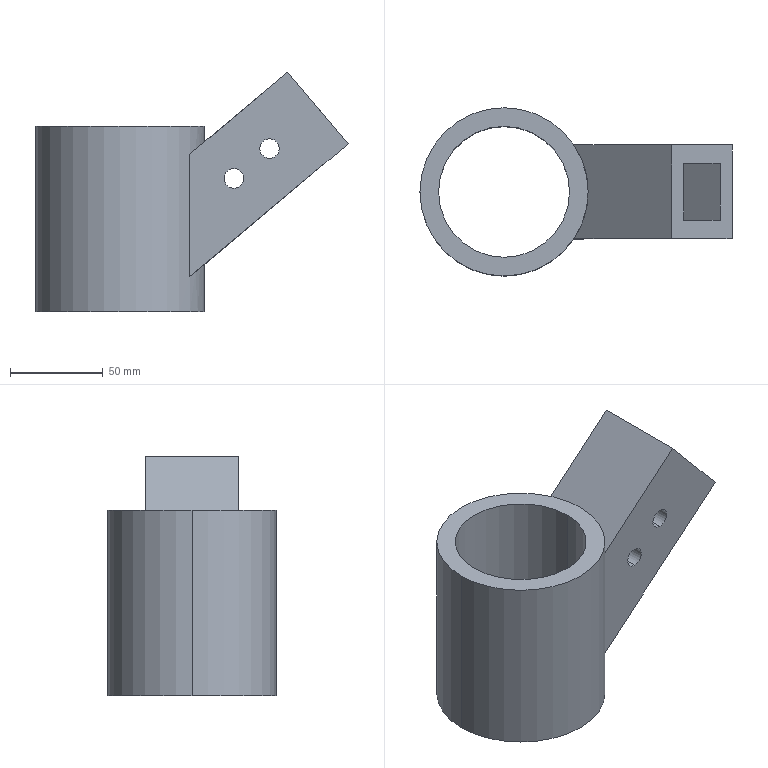Part | SolidWorks | features MirrorStock 1 | 1 solid | 24 faces | box 167.949 x 90.5 x 129.102 mm | volume 386069 mm3 | cylinder 13 | plane 11 | commonest cylinder face diameters 10.5 x8 90.5 x3 70.5 x2
STEP:
#1=CARTESIAN_POINT('',(80.423,15.25,43.155));
#2=VERTEX_POINT('',#1);
#3=CARTESIAN_POINT('',(80.423,15.25,32.655));
#4=VERTEX_POINT('',#3);
#5=CARTESIAN_POINT('',(80.423,15.25,37.905));
#6=DIRECTION('',(0.,1.,0.));
#7=DIRECTION('',(0.,0.,1.));
#8=AXIS2_PLACEMENT_3D('',#5,#6,#7);
#9=CIRCLE('',#8,5.25);
#10=EDGE_CURVE('',#2,#4,#9,.T.);
#11=ORIENTED_EDGE('',*,*,#10,.F.);
#12=CARTESIAN_POINT('',(80.423,25.25,43.155));
#13=VERTEX_POINT('',#12);
#14=CARTESIAN_POINT('',(80.423,-57.25,43.155));
#15=DIRECTION('',(0.,1.,0.));
#16=VECTOR('',#15,1000.);
#17=LINE('',#14,#16);
#18=EDGE_CURVE('',#2,#13,#17,.T.);
#19=ORIENTED_EDGE('',*,*,#18,.T.);
#20=CARTESIAN_POINT('',(80.423,25.25,32.655));
#21=VERTEX_POINT('',#20);
#22=CARTESIAN_POINT('',(80.423,25.25,37.905));
#23=DIRECTION('',(0.,1.,0.));
#24=DIRECTION('',(0.,0.,1.));
#25=AXIS2_PLACEMENT_3D('',#22,#23,#24);
#26=CIRCLE('',#25,5.25);
#27=EDGE_CURVE('',#13,#21,#26,.T.);
#28=ORIENTED_EDGE('',*,*,#27,.T.);
#29=CARTESIAN_POINT('',(80.423,-57.25,32.655));
#30=DIRECTION('',(0.,1.,0.));
#31=VECTOR('',#30,1000.);
#32=LINE('',#29,#31);
#33=EDGE_CURVE('',#4,#21,#32,.T.);
#34=ORIENTED_EDGE('',*,*,#33,.F.);
#35=EDGE_LOOP('',(#11,#19,#28,#34));
#36=FACE_OUTER_BOUND('',#35,.T.);
#37=CARTESIAN_POINT('',(80.423,-57.25,37.905));
#38=DIRECTION('',(0.,1.,0.));
#39=DIRECTION('',(0.,0.,-1.));
#40=AXIS2_PLACEMENT_3D('',#37,#38,#39);
#41=CYLINDRICAL_SURFACE('',#40,5.25);
#42=ADVANCED_FACE('',(#36),#41,.F.);
#43=CARTESIAN_POINT('',(61.272,15.25,27.085));
#44=VERTEX_POINT('',#43);
#45=CARTESIAN_POINT('',(61.272,15.25,16.585));
#46=VERTEX_POINT('',#45);
#47=CARTESIAN_POINT('',(61.272,15.25,21.835));
#48=DIRECTION('',(0.,1.,0.));
#49=DIRECTION('',(0.,0.,1.));
#50=AXIS2_PLACEMENT_3D('',#47,#48,#49);
#51=CIRCLE('',#50,5.25);
#52=EDGE_CURVE('',#44,#46,#51,.T.);
#53=ORIENTED_EDGE('',*,*,#52,.F.);
#54=CARTESIAN_POINT('',(61.272,25.25,27.085));
#55=VERTEX_POINT('',#54);
#56=CARTESIAN_POINT('',(61.272,-57.25,27.085));
#57=DIRECTION('',(0.,1.,0.));
#58=VECTOR('',#57,1000.);
#59=LINE('',#56,#58);
#60=EDGE_CURVE('',#44,#55,#59,.T.);
#61=ORIENTED_EDGE('',*,*,#60,.T.);
#62=CARTESIAN_POINT('',(61.272,25.25,16.585));
#63=VERTEX_POINT('',#62);
#64=CARTESIAN_POINT('',(61.272,25.25,21.835));
#65=DIRECTION('',(0.,1.,0.));
#66=DIRECTION('',(0.,0.,1.));
#67=AXIS2_PLACEMENT_3D('',#64,#65,#66);
#68=CIRCLE('',#67,5.25);
#69=EDGE_CURVE('',#55,#63,#68,.T.);
#70=ORIENTED_EDGE('',*,*,#69,.T.);
#71=CARTESIAN_POINT('',(61.272,-57.25,16.585));
#72=DIRECTION('',(0.,1.,0.));
#73=VECTOR('',#72,1000.);
#74=LINE('',#71,#73);
#75=EDGE_CURVE('',#46,#63,#74,.T.);
#76=ORIENTED_EDGE('',*,*,#75,.F.);
#77=EDGE_LOOP('',(#53,#61,#70,#76));
#78=FACE_OUTER_BOUND('',#77,.T.);
#79=CARTESIAN_POINT('',(61.272,-57.25,21.835));
#80=DIRECTION('',(0.,1.,0.));
#81=DIRECTION('',(0.,0.,-1.));
#82=AXIS2_PLACEMENT_3D('',#79,#80,#81);
#83=CYLINDRICAL_SURFACE('',#82,5.25);
#84=ADVANCED_FACE('',(#78),#83,.F.);
#85=CARTESIAN_POINT('',(80.423,-25.25,32.655));
#86=VERTEX_POINT('',#85);
#87=CARTESIAN_POINT('',(80.423,-25.25,43.155));
#88=VERTEX_POINT('',#87);
#89=CARTESIAN_POINT('',(80.423,-25.25,37.905));
#90=DIRECTION('',(0.,-1.,0.));
#91=DIRECTION('',(0.,0.,-1.));
#92=AXIS2_PLACEMENT_3D('',#89,#90,#91);
#93=CIRCLE('',#92,5.25);
#94=EDGE_CURVE('',#86,#88,#93,.T.);
#95=ORIENTED_EDGE('',*,*,#94,.T.);
#96=CARTESIAN_POINT('',(80.423,-15.25,43.155));
#97=VERTEX_POINT('',#96);
#98=CARTESIAN_POINT('',(80.423,-57.25,43.155));
#99=DIRECTION('',(0.,1.,0.));
#100=VECTOR('',#99,1000.);
#101=LINE('',#98,#100);
#102=EDGE_CURVE('',#88,#97,#101,.T.);
#103=ORIENTED_EDGE('',*,*,#102,.T.);
#104=CARTESIAN_POINT('',(80.423,-15.25,32.655));
#105=VERTEX_POINT('',#104);
#106=CARTESIAN_POINT('',(80.423,-15.25,37.905));
#107=DIRECTION('',(0.,-1.,0.));
#108=DIRECTION('',(0.,0.,-1.));
#109=AXIS2_PLACEMENT_3D('',#106,#107,#108);
#110=CIRCLE('',#109,5.25);
#111=EDGE_CURVE('',#105,#97,#110,.T.);
#112=ORIENTED_EDGE('',*,*,#111,.F.);
#113=CARTESIAN_POINT('',(80.423,-57.25,32.655));
#114=DIRECTION('',(0.,1.,0.));
#115=VECTOR('',#114,1000.);
#116=LINE('',#113,#115);
#117=EDGE_CURVE('',#86,#105,#116,.T.);
#118=ORIENTED_EDGE('',*,*,#117,.F.);
#119=EDGE_LOOP('',(#95,#103,#112,#118));
#120=FACE_OUTER_BOUND('',#119,.T.);
#121=CARTESIAN_POINT('',(80.423,-57.25,37.905));
#122=DIRECTION('',(0.,1.,0.));
#123=DIRECTION('',(0.,0.,-1.));
#124=AXIS2_PLACEMENT_3D('',#121,#122,#123);
#125=CYLINDRICAL_SURFACE('',#124,5.25);
#126=ADVANCED_FACE('',(#120),#125,.F.);
#127=CARTESIAN_POINT('',(61.272,-25.25,16.585));
#128=VERTEX_POINT('',#127);
#129=CARTESIAN_POINT('',(61.272,-25.25,27.085));
#130=VERTEX_POINT('',#129);
#131=CARTESIAN_POINT('',(61.272,-25.25,21.835));
#132=DIRECTION('',(0.,-1.,0.));
#133=DIRECTION('',(0.,0.,-1.));
#134=AXIS2_PLACEMENT_3D('',#131,#132,#133);
#135=CIRCLE('',#134,5.25);
#136=EDGE_CURVE('',#128,#130,#135,.T.);
#137=ORIENTED_EDGE('',*,*,#136,.T.);
#138=CARTESIAN_POINT('',(61.272,-15.25,27.085));
#139=VERTEX_POINT('',#138);
#140=CARTESIAN_POINT('',(61.272,-57.25,27.085));
#141=DIRECTION('',(0.,1.,0.));
#142=VECTOR('',#141,1000.);
#143=LINE('',#140,#142);
#144=EDGE_CURVE('',#130,#139,#143,.T.);
#145=ORIENTED_EDGE('',*,*,#144,.T.);
#146=CARTESIAN_POINT('',(61.272,-15.25,16.585));
#147=VERTEX_POINT('',#146);
#148=CARTESIAN_POINT('',(61.272,-15.25,21.835));
#149=DIRECTION('',(0.,-1.,0.));
#150=DIRECTION('',(0.,0.,-1.));
#151=AXIS2_PLACEMENT_3D('',#148,#149,#150);
#152=CIRCLE('',#151,5.25);
#153=EDGE_CURVE('',#147,#139,#152,.T.);
#154=ORIENTED_EDGE('',*,*,#153,.F.);
#155=CARTESIAN_POINT('',(61.272,-57.25,16.585));
#156=DIRECTION('',(0.,1.,0.));
#157=VECTOR('',#156,1000.);
#158=LINE('',#155,#157);
#159=EDGE_CURVE('',#128,#147,#158,.T.);
#160=ORIENTED_EDGE('',*,*,#159,.F.);
#161=EDGE_LOOP('',(#137,#145,#154,#160));
#162=FACE_OUTER_BOUND('',#161,.T.);
#163=CARTESIAN_POINT('',(61.272,-57.25,21.835));
#164=DIRECTION('',(0.,1.,0.));
#165=DIRECTION('',(0.,0.,-1.));
#166=AXIS2_PLACEMENT_3D('',#163,#164,#165);
#167=CYLINDRICAL_SURFACE('',#166,5.25);
#168=ADVANCED_FACE('',(#162),#167,.F.);
#169=CARTESIAN_POINT('',(35.25,0.,-50.));
#170=VERTEX_POINT('',#169);
#171=CARTESIAN_POINT('',(-35.25,0.,-50.));
#172=VERTEX_POINT('',#171);
#173=CARTESIAN_POINT('',(0.,0.,-50.));
#174=DIRECTION('',(0.,0.,1.));
#175=DIRECTION('',(1.,0.,0.));
#176=AXIS2_PLACEMENT_3D('',#173,#174,#175);
#177=CIRCLE('',#176,35.25);
#178=EDGE_CURVE('',#170,#172,#177,.T.);
#179=ORIENTED_EDGE('',*,*,#178,.F.);
#180=CARTESIAN_POINT('',(35.25,0.,50.));
#181=VERTEX_POINT('',#180);
#182=CARTESIAN_POINT('',(35.25,0.,-50.));
#183=DIRECTION('',(0.,0.,1.));
#184=VECTOR('',#183,1000.);
#185=LINE('',#182,#184);
#186=EDGE_CURVE('',#170,#181,#185,.T.);
#187=ORIENTED_EDGE('',*,*,#186,.T.);
#188=CARTESIAN_POINT('',(-35.25,0.,50.));
#189=VERTEX_POINT('',#188);
#190=CARTESIAN_POINT('',(0.,0.,50.));
#191=DIRECTION('',(0.,0.,1.));
#192=DIRECTION('',(1.,0.,0.));
#193=AXIS2_PLACEMENT_3D('',#190,#191,#192);
#194=CIRCLE('',#193,35.25);
#195=EDGE_CURVE('',#181,#189,#194,.T.);
#196=ORIENTED_EDGE('',*,*,#195,.T.);
#197=CARTESIAN_POINT('',(-35.25,0.,-50.));
#198=DIRECTION('',(0.,0.,1.));
#199=VECTOR('',#198,1000.);
#200=LINE('',#197,#199);
#201=EDGE_CURVE('',#172,#189,#200,.T.);
#202=ORIENTED_EDGE('',*,*,#201,.F.);
#203=EDGE_LOOP('',(#179,#187,#196,#202));
#204=FACE_OUTER_BOUND('',#203,.T.);
#205=CARTESIAN_POINT('',(0.,0.,-50.));
#206=DIRECTION('',(0.,0.,1.));
#207=DIRECTION('',(-1.,0.,0.));
#208=AXIS2_PLACEMENT_3D('',#205,#206,#207);
#209=CYLINDRICAL_SURFACE('',#208,35.25);
#210=ADVANCED_FACE('',(#204),#209,.F.);
#211=CARTESIAN_POINT('',(-45.25,0.,-50.));
#212=VERTEX_POINT('',#211);
#213=CARTESIAN_POINT('',(45.25,0.,-50.));
#214=VERTEX_POINT('',#213);
#215=CARTESIAN_POINT('',(0.,0.,-50.));
#216=DIRECTION('',(0.,0.,1.));
#217=DIRECTION('',(1.,0.,0.));
#218=AXIS2_PLACEMENT_3D('',#215,#216,#217);
#219=CIRCLE('',#218,45.25);
#220=EDGE_CURVE('',#212,#214,#219,.T.);
#221=ORIENTED_EDGE('',*,*,#220,.T.);
#222=CARTESIAN_POINT('',(45.25,0.,-24.571));
#223=VERTEX_POINT('',#222);
#224=CARTESIAN_POINT('',(45.25,0.,-50.));
#225=DIRECTION('',(0.,0.,1.));
#226=VECTOR('',#225,1000.);
#227=LINE('',#224,#226);
#228=EDGE_CURVE('',#214,#223,#227,.T.);
#229=ORIENTED_EDGE('',*,*,#228,.T.);
#230=CARTESIAN_POINT('',(37.55,-25.25,-31.032));
#231=VERTEX_POINT('',#230);
#232=CARTESIAN_POINT('',(45.25,0.,-24.571));
#233=CARTESIAN_POINT('',(45.25,-9.062,-24.571));
#234=CARTESIAN_POINT('',(42.607,-17.73,-26.789));
#235=CARTESIAN_POINT('',(37.55,-25.25,-31.032));
#236=(BOUNDED_CURVE()B_SPLINE_CURVE(3,(#232,#233,#234,#235),.UNSPECIFIED.,.F.,.T.)B_SPLINE_CURVE_WITH_KNOTS((4,4),(0.,0.592),.UNSPECIFIED.)CURVE()GEOMETRIC_REPRESENTATION_ITEM()RATIONAL_B_SPLINE_CURVE((1.,0.971,0.971,1.))REPRESENTATION_ITEM(''));
#237=EDGE_CURVE('',#223,#231,#236,.T.);
#238=ORIENTED_EDGE('',*,*,#237,.T.);
#239=CARTESIAN_POINT('',(37.55,-25.25,34.891));
#240=VERTEX_POINT('',#239);
#241=CARTESIAN_POINT('',(37.55,-25.25,-50.));
#242=DIRECTION('',(0.,0.,1.));
#243=VECTOR('',#242,1000.);
#244=LINE('',#241,#243);
#245=EDGE_CURVE('',#231,#240,#244,.T.);
#246=ORIENTED_EDGE('',*,*,#245,.T.);
#247=CARTESIAN_POINT('',(45.25,0.,41.353));
#248=VERTEX_POINT('',#247);
#249=CARTESIAN_POINT('',(45.25,0.,41.353));
#250=CARTESIAN_POINT('',(45.25,-9.062,41.353));
#251=CARTESIAN_POINT('',(42.607,-17.73,39.135));
#252=CARTESIAN_POINT('',(37.55,-25.25,34.891));
#253=(BOUNDED_CURVE()B_SPLINE_CURVE(3,(#249,#250,#251,#252),.UNSPECIFIED.,.F.,.T.)B_SPLINE_CURVE_WITH_KNOTS((4,4),(0.,0.592),.UNSPECIFIED.)CURVE()GEOMETRIC_REPRESENTATION_ITEM()RATIONAL_B_SPLINE_CURVE((1.,0.971,0.971,1.))REPRESENTATION_ITEM(''));
#254=EDGE_CURVE('',#248,#240,#253,.T.);
#255=ORIENTED_EDGE('',*,*,#254,.F.);
#256=CARTESIAN_POINT('',(45.25,0.,50.));
#257=VERTEX_POINT('',#256);
#258=CARTESIAN_POINT('',(45.25,0.,-50.));
#259=DIRECTION('',(0.,0.,1.));
#260=VECTOR('',#259,1000.);
#261=LINE('',#258,#260);
#262=EDGE_CURVE('',#248,#257,#261,.T.);
#263=ORIENTED_EDGE('',*,*,#262,.T.);
#264=CARTESIAN_POINT('',(-45.25,0.,50.));
#265=VERTEX_POINT('',#264);
#266=CARTESIAN_POINT('',(0.,0.,50.));
#267=DIRECTION('',(0.,0.,1.));
#268=DIRECTION('',(1.,0.,0.));
#269=AXIS2_PLACEMENT_3D('',#266,#267,#268);
#270=CIRCLE('',#269,45.25);
#271=EDGE_CURVE('',#265,#257,#270,.T.);
#272=ORIENTED_EDGE('',*,*,#271,.F.);
#273=CARTESIAN_POINT('',(-45.25,0.,-50.));
#274=DIRECTION('',(0.,0.,1.));
#275=VECTOR('',#274,1000.);
#276=LINE('',#273,#275);
#277=EDGE_CURVE('',#212,#265,#276,.T.);
#278=ORIENTED_EDGE('',*,*,#277,.F.);
#279=EDGE_LOOP('',(#221,#229,#238,#246,#255,#263,#272,#278));
#280=FACE_OUTER_BOUND('',#279,.T.);
#281=CARTESIAN_POINT('',(0.,0.,-50.));
#282=DIRECTION('',(0.,0.,1.));
#283=DIRECTION('',(-1.,0.,0.));
#284=AXIS2_PLACEMENT_3D('',#281,#282,#283);
#285=CYLINDRICAL_SURFACE('',#284,45.25);
#286=ADVANCED_FACE('',(#280),#285,.T.);
#287=ORIENTED_EDGE('',*,*,#228,.F.);
#288=CARTESIAN_POINT('',(0.,0.,-50.));
#289=DIRECTION('',(0.,0.,1.));
#290=DIRECTION('',(1.,0.,0.));
#291=AXIS2_PLACEMENT_3D('',#288,#289,#290);
#292=CIRCLE('',#291,45.25);
#293=EDGE_CURVE('',#214,#212,#292,.T.);
#294=ORIENTED_EDGE('',*,*,#293,.T.);
#295=ORIENTED_EDGE('',*,*,#277,.T.);
#296=CARTESIAN_POINT('',(0.,0.,50.));
#297=DIRECTION('',(0.,0.,1.));
#298=DIRECTION('',(1.,0.,0.));
#299=AXIS2_PLACEMENT_3D('',#296,#297,#298);
#300=CIRCLE('',#299,45.25);
#301=EDGE_CURVE('',#257,#265,#300,.T.);
#302=ORIENTED_EDGE('',*,*,#301,.F.);
#303=ORIENTED_EDGE('',*,*,#262,.F.);
#304=CARTESIAN_POINT('',(37.55,25.25,34.891));
#305=VERTEX_POINT('',#304);
#306=CARTESIAN_POINT('',(37.55,25.25,34.891));
#307=CARTESIAN_POINT('',(42.607,17.73,39.135));
#308=CARTESIAN_POINT('',(45.25,9.062,41.353));
#309=CARTESIAN_POINT('',(45.25,0.,41.353));
#310=(BOUNDED_CURVE()B_SPLINE_CURVE(3,(#306,#307,#308,#309),.UNSPECIFIED.,.F.,.T.)B_SPLINE_CURVE_WITH_KNOTS((4,4),(5.691,6.283),.UNSPECIFIED.)CURVE()GEOMETRIC_REPRESENTATION_ITEM()RATIONAL_B_SPLINE_CURVE((1.,0.971,0.971,1.))REPRESENTATION_ITEM(''));
#311=EDGE_CURVE('',#305,#248,#310,.T.);
#312=ORIENTED_EDGE('',*,*,#311,.F.);
#313=CARTESIAN_POINT('',(37.55,25.25,-31.032));
#314=VERTEX_POINT('',#313);
#315=CARTESIAN_POINT('',(37.55,25.25,-50.));
#316=DIRECTION('',(0.,0.,-1.));
#317=VECTOR('',#316,1000.);
#318=LINE('',#315,#317);
#319=EDGE_CURVE('',#305,#314,#318,.T.);
#320=ORIENTED_EDGE('',*,*,#319,.T.);
#321=CARTESIAN_POINT('',(37.55,25.25,-31.032));
#322=CARTESIAN_POINT('',(42.607,17.73,-26.789));
#323=CARTESIAN_POINT('',(45.25,9.062,-24.571));
#324=CARTESIAN_POINT('',(45.25,0.,-24.571));
#325=(BOUNDED_CURVE()B_SPLINE_CURVE(3,(#321,#322,#323,#324),.UNSPECIFIED.,.F.,.T.)B_SPLINE_CURVE_WITH_KNOTS((4,4),(5.691,6.283),.UNSPECIFIED.)CURVE()GEOMETRIC_REPRESENTATION_ITEM()RATIONAL_B_SPLINE_CURVE((1.,0.971,0.971,1.))REPRESENTATION_ITEM(''));
#326=EDGE_CURVE('',#314,#223,#325,.T.);
#327=ORIENTED_EDGE('',*,*,#326,.T.);
#328=EDGE_LOOP('',(#287,#294,#295,#302,#303,#312,#320,#327));
#329=FACE_OUTER_BOUND('',#328,.T.);
#330=CARTESIAN_POINT('',(0.,0.,-50.));
#331=DIRECTION('',(0.,0.,1.));
#332=DIRECTION('',(-1.,0.,0.));
#333=AXIS2_PLACEMENT_3D('',#330,#331,#332);
#334=CYLINDRICAL_SURFACE('',#333,45.25);
#335=ADVANCED_FACE('',(#329),#334,.T.);
#336=CARTESIAN_POINT('',(42.603,15.25,-13.738));
#337=VERTEX_POINT('',#336);
#338=CARTESIAN_POINT('',(42.603,-15.25,-13.738));
#339=VERTEX_POINT('',#338);
#340=CARTESIAN_POINT('',(42.603,15.25,-13.738));
#341=CARTESIAN_POINT('',(46.168,5.29,-10.746));
#342=CARTESIAN_POINT('',(46.168,-5.29,-10.746));
#343=CARTESIAN_POINT('',(42.603,-15.25,-13.738));
#344=(BOUNDED_CURVE()B_SPLINE_CURVE(3,(#340,#341,#342,#343),.UNSPECIFIED.,.F.,.T.)B_SPLINE_CURVE_WITH_KNOTS((4,4),(5.939,6.627),.UNSPECIFIED.)CURVE()GEOMETRIC_REPRESENTATION_ITEM()RATIONAL_B_SPLINE_CURVE((1.,0.961,0.961,1.))REPRESENTATION_ITEM(''));
#345=EDGE_CURVE('',#337,#339,#344,.T.);
#346=ORIENTED_EDGE('',*,*,#345,.F.);
#347=CARTESIAN_POINT('',(42.603,15.25,26.077));
#348=VERTEX_POINT('',#347);
#349=CARTESIAN_POINT('',(42.603,15.25,-50.));
#350=DIRECTION('',(0.,0.,-1.));
#351=VECTOR('',#350,1000.);
#352=LINE('',#349,#351);
#353=EDGE_CURVE('',#348,#337,#352,.T.);
#354=ORIENTED_EDGE('',*,*,#353,.F.);
#355=CARTESIAN_POINT('',(42.603,-15.25,26.077));
#356=VERTEX_POINT('',#355);
#357=CARTESIAN_POINT('',(42.603,15.25,26.077));
#358=CARTESIAN_POINT('',(46.168,5.29,29.069));
#359=CARTESIAN_POINT('',(46.168,-5.29,29.069));
#360=CARTESIAN_POINT('',(42.603,-15.25,26.077));
#361=(BOUNDED_CURVE()B_SPLINE_CURVE(3,(#357,#358,#359,#360),.UNSPECIFIED.,.F.,.T.)B_SPLINE_CURVE_WITH_KNOTS((4,4),(5.939,6.627),.UNSPECIFIED.)CURVE()GEOMETRIC_REPRESENTATION_ITEM()RATIONAL_B_SPLINE_CURVE((1.,0.961,0.961,1.))REPRESENTATION_ITEM(''));
#362=EDGE_CURVE('',#348,#356,#361,.T.);
#363=ORIENTED_EDGE('',*,*,#362,.T.);
#364=CARTESIAN_POINT('',(42.603,-15.25,-50.));
#365=DIRECTION('',(0.,0.,1.));
#366=VECTOR('',#365,1000.);
#367=LINE('',#364,#366);
#368=EDGE_CURVE('',#339,#356,#367,.T.);
#369=ORIENTED_EDGE('',*,*,#368,.F.);
#370=EDGE_LOOP('',(#346,#354,#363,#369));
#371=FACE_OUTER_BOUND('',#370,.T.);
#372=CARTESIAN_POINT('',(0.,0.,-50.));
#373=DIRECTION('',(0.,0.,1.));
#374=DIRECTION('',(-1.,0.,0.));
#375=AXIS2_PLACEMENT_3D('',#372,#373,#374);
#376=CYLINDRICAL_SURFACE('',#375,45.25);
#377=ADVANCED_FACE('',(#371),#376,.T.);
#378=ORIENTED_EDGE('',*,*,#220,.F.);
#379=ORIENTED_EDGE('',*,*,#293,.F.);
#380=EDGE_LOOP('',(#378,#379));
#381=FACE_OUTER_BOUND('',#380,.T.);
#382=CARTESIAN_POINT('',(0.,0.,-50.));
#383=DIRECTION('',(0.,0.,1.));
#384=DIRECTION('',(1.,0.,0.));
#385=AXIS2_PLACEMENT_3D('',#382,#383,#384);
#386=CIRCLE('',#385,35.25);
#387=EDGE_CURVE('',#172,#170,#386,.T.);
#388=ORIENTED_EDGE('',*,*,#387,.T.);
#389=ORIENTED_EDGE('',*,*,#178,.T.);
#390=EDGE_LOOP('',(#388,#389));
#391=FACE_BOUND('',#390,.T.);
#392=CARTESIAN_POINT('',(0.,0.,-50.));
#393=DIRECTION('',(0.,0.,-1.));
#394=DIRECTION('',(1.,0.,0.));
#395=AXIS2_PLACEMENT_3D('',#392,#393,#394);
#396=PLANE('',#395);
#397=ADVANCED_FACE('',(#381,#391),#396,.T.);
#398=ORIENTED_EDGE('',*,*,#271,.T.);
#399=ORIENTED_EDGE('',*,*,#301,.T.);
#400=EDGE_LOOP('',(#398,#399));
#401=FACE_OUTER_BOUND('',#400,.T.);
#402=CARTESIAN_POINT('',(0.,0.,50.));
#403=DIRECTION('',(0.,0.,1.));
#404=DIRECTION('',(1.,0.,0.));
#405=AXIS2_PLACEMENT_3D('',#402,#403,#404);
#406=CIRCLE('',#405,35.25);
#407=EDGE_CURVE('',#189,#181,#406,.T.);
#408=ORIENTED_EDGE('',*,*,#407,.F.);
#409=ORIENTED_EDGE('',*,*,#195,.F.);
#410=EDGE_LOOP('',(#408,#409));
#411=FACE_BOUND('',#410,.T.);
#412=CARTESIAN_POINT('',(0.,0.,50.));
#413=DIRECTION('',(0.,0.,-1.));
#414=DIRECTION('',(1.,0.,0.));
#415=AXIS2_PLACEMENT_3D('',#412,#413,#414);
#416=PLANE('',#415);
#417=ADVANCED_FACE('',(#401,#411),#416,.F.);
#418=ORIENTED_EDGE('',*,*,#186,.F.);
#419=ORIENTED_EDGE('',*,*,#387,.F.);
#420=ORIENTED_EDGE('',*,*,#201,.T.);
#421=ORIENTED_EDGE('',*,*,#407,.T.);
#422=EDGE_LOOP('',(#418,#419,#420,#421));
#423=FACE_OUTER_BOUND('',#422,.T.);
#424=CARTESIAN_POINT('',(0.,0.,-50.));
#425=DIRECTION('',(0.,0.,1.));
#426=DIRECTION('',(-1.,0.,0.));
#427=AXIS2_PLACEMENT_3D('',#424,#425,#426);
#428=CYLINDRICAL_SURFACE('',#427,35.25);
#429=ADVANCED_FACE('',(#423),#428,.F.);
#430=ORIENTED_EDGE('',*,*,#311,.T.);
#431=ORIENTED_EDGE('',*,*,#254,.T.);
#432=CARTESIAN_POINT('',(90.238,-25.25,79.102));
#433=VERTEX_POINT('',#432);
#434=CARTESIAN_POINT('',(35.25,-25.25,32.962));
#435=DIRECTION('',(-0.766,0.,-0.6428));
#436=VECTOR('',#435,1000.);
#437=LINE('',#434,#436);
#438=EDGE_CURVE('',#433,#240,#437,.T.);
#439=ORIENTED_EDGE('',*,*,#438,.F.);
#440=CARTESIAN_POINT('',(90.238,25.25,79.102));
#441=VERTEX_POINT('',#440);
#442=CARTESIAN_POINT('',(90.238,15.25,79.102));
#443=DIRECTION('',(0.,-1.,0.));
#444=VECTOR('',#443,1000.);
#445=LINE('',#442,#444);
#446=EDGE_CURVE('',#441,#433,#445,.T.);
#447=ORIENTED_EDGE('',*,*,#446,.F.);
#448=CARTESIAN_POINT('',(35.25,25.25,32.962));
#449=DIRECTION('',(-0.766,0.,-0.6428));
#450=VECTOR('',#449,1000.);
#451=LINE('',#448,#450);
#452=EDGE_CURVE('',#441,#305,#451,.T.);
#453=ORIENTED_EDGE('',*,*,#452,.T.);
#454=EDGE_LOOP('',(#430,#431,#439,#447,#453));
#455=FACE_OUTER_BOUND('',#454,.T.);
#456=CARTESIAN_POINT('',(-1.666,15.25,1.985));
#457=DIRECTION('',(-0.6428,0.,0.766));
#458=DIRECTION('',(-0.766,0.,-0.6428));
#459=AXIS2_PLACEMENT_3D('',#456,#457,#458);
#460=PLANE('',#459);
#461=ADVANCED_FACE('',(#455),#460,.T.);
#462=CARTESIAN_POINT('',(96.666,15.25,71.441));
#463=VERTEX_POINT('',#462);
#464=CARTESIAN_POINT('',(4.762,15.25,-5.675));
#465=DIRECTION('',(0.766,0.,0.6428));
#466=VECTOR('',#465,1000.);
#467=LINE('',#464,#466);
#468=EDGE_CURVE('',#348,#463,#467,.T.);
#469=ORIENTED_EDGE('',*,*,#468,.T.);
#470=CARTESIAN_POINT('',(96.666,-15.25,71.441));
#471=VERTEX_POINT('',#470);
#472=CARTESIAN_POINT('',(96.666,15.25,71.441));
#473=DIRECTION('',(0.,-1.,0.));
#474=VECTOR('',#473,1000.);
#475=LINE('',#472,#474);
#476=EDGE_CURVE('',#463,#471,#475,.T.);
#477=ORIENTED_EDGE('',*,*,#476,.T.);
#478=CARTESIAN_POINT('',(4.762,-15.25,-5.675));
#479=DIRECTION('',(0.766,0.,0.6428));
#480=VECTOR('',#479,1000.);
#481=LINE('',#478,#480);
#482=EDGE_CURVE('',#356,#471,#481,.T.);
#483=ORIENTED_EDGE('',*,*,#482,.F.);
#484=ORIENTED_EDGE('',*,*,#362,.F.);
#485=EDGE_LOOP('',(#469,#477,#483,#484));
#486=FACE_OUTER_BOUND('',#485,.T.);
#487=CARTESIAN_POINT('',(4.762,15.25,-5.675));
#488=DIRECTION('',(-0.6428,0.,0.766));
#489=DIRECTION('',(-0.766,0.,-0.6428));
#490=AXIS2_PLACEMENT_3D('',#487,#488,#489);
#491=PLANE('',#490);
#492=ADVANCED_FACE('',(#486),#491,.F.);
#493=ORIENTED_EDGE('',*,*,#476,.F.);
#494=CARTESIAN_POINT('',(116.271,15.25,48.077));
#495=VERTEX_POINT('',#494);
#496=CARTESIAN_POINT('',(90.238,15.25,79.102));
#497=DIRECTION('',(-0.6428,0.,0.766));
#498=VECTOR('',#497,1000.);
#499=LINE('',#496,#498);
#500=EDGE_CURVE('',#495,#463,#499,.T.);
#501=ORIENTED_EDGE('',*,*,#500,.F.);
#502=CARTESIAN_POINT('',(116.271,-15.25,48.077));
#503=VERTEX_POINT('',#502);
#504=CARTESIAN_POINT('',(116.271,15.25,48.077));
#505=DIRECTION('',(0.,-1.,0.));
#506=VECTOR('',#505,1000.);
#507=LINE('',#504,#506);
#508=EDGE_CURVE('',#495,#503,#507,.T.);
#509=ORIENTED_EDGE('',*,*,#508,.T.);
#510=CARTESIAN_POINT('',(90.238,-15.25,79.102));
#511=DIRECTION('',(-0.6428,0.,0.766));
#512=VECTOR('',#511,1000.);
#513=LINE('',#510,#512);
#514=EDGE_CURVE('',#503,#471,#513,.T.);
#515=ORIENTED_EDGE('',*,*,#514,.T.);
#516=EDGE_LOOP('',(#493,#501,#509,#515));
#517=FACE_BOUND('',#516,.T.);
#518=CARTESIAN_POINT('',(122.699,-25.25,40.417));
#519=VERTEX_POINT('',#518);
#520=CARTESIAN_POINT('',(90.238,-25.25,79.102));
#521=DIRECTION('',(-0.6428,0.,0.766));
#522=VECTOR('',#521,1000.);
#523=LINE('',#520,#522);
#524=EDGE_CURVE('',#519,#433,#523,.T.);
#525=ORIENTED_EDGE('',*,*,#524,.F.);
#526=CARTESIAN_POINT('',(122.699,25.25,40.417));
#527=VERTEX_POINT('',#526);
#528=CARTESIAN_POINT('',(122.699,15.25,40.417));
#529=DIRECTION('',(0.,-1.,0.));
#530=VECTOR('',#529,1000.);
#531=LINE('',#528,#530);
#532=EDGE_CURVE('',#527,#519,#531,.T.);
#533=ORIENTED_EDGE('',*,*,#532,.F.);
#534=CARTESIAN_POINT('',(90.238,25.25,79.102));
#535=DIRECTION('',(-0.6428,0.,0.766));
#536=VECTOR('',#535,1000.);
#537=LINE('',#534,#536);
#538=EDGE_CURVE('',#527,#441,#537,.T.);
#539=ORIENTED_EDGE('',*,*,#538,.T.);
#540=ORIENTED_EDGE('',*,*,#446,.T.);
#541=EDGE_LOOP('',(#525,#533,#539,#540));
#542=FACE_OUTER_BOUND('',#541,.T.);
#543=CARTESIAN_POINT('',(91.904,15.25,77.117));
#544=DIRECTION('',(0.766,0.,0.6428));
#545=DIRECTION('',(-0.6428,0.,0.766));
#546=AXIS2_PLACEMENT_3D('',#543,#544,#545);
#547=PLANE('',#546);
#548=ADVANCED_FACE('',(#517,#542),#547,.T.);
#549=ORIENTED_EDGE('',*,*,#345,.T.);
#550=CARTESIAN_POINT('',(24.367,-15.25,-29.039));
#551=DIRECTION('',(0.766,0.,0.6428));
#552=VECTOR('',#551,1000.);
#553=LINE('',#550,#552);
#554=EDGE_CURVE('',#339,#503,#553,.T.);
#555=ORIENTED_EDGE('',*,*,#554,.T.);
#556=ORIENTED_EDGE('',*,*,#508,.F.);
#557=CARTESIAN_POINT('',(24.367,15.25,-29.039));
#558=DIRECTION('',(0.766,0.,0.6428));
#559=VECTOR('',#558,1000.);
#560=LINE('',#557,#559);
#561=EDGE_CURVE('',#337,#495,#560,.T.);
#562=ORIENTED_EDGE('',*,*,#561,.F.);
#563=EDGE_LOOP('',(#549,#555,#556,#562));
#564=FACE_OUTER_BOUND('',#563,.T.);
#565=CARTESIAN_POINT('',(24.367,15.25,-29.039));
#566=DIRECTION('',(-0.6428,0.,0.766));
#567=DIRECTION('',(-0.766,0.,-0.6428));
#568=AXIS2_PLACEMENT_3D('',#565,#566,#567);
#569=PLANE('',#568);
#570=ADVANCED_FACE('',(#564),#569,.T.);
#571=ORIENTED_EDGE('',*,*,#532,.T.);
#572=CARTESIAN_POINT('',(122.699,-25.25,40.417));
#573=DIRECTION('',(0.766,0.,0.6428));
#574=VECTOR('',#573,1000.);
#575=LINE('',#572,#574);
#576=EDGE_CURVE('',#231,#519,#575,.T.);
#577=ORIENTED_EDGE('',*,*,#576,.F.);
#578=ORIENTED_EDGE('',*,*,#237,.F.);
#579=ORIENTED_EDGE('',*,*,#326,.F.);
#580=CARTESIAN_POINT('',(122.699,25.25,40.417));
#581=DIRECTION('',(0.766,0.,0.6428));
#582=VECTOR('',#581,1000.);
#583=LINE('',#580,#582);
#584=EDGE_CURVE('',#314,#527,#583,.T.);
#585=ORIENTED_EDGE('',*,*,#584,.T.);
#586=EDGE_LOOP('',(#571,#577,#578,#579,#585));
#587=FACE_OUTER_BOUND('',#586,.T.);
#588=CARTESIAN_POINT('',(30.795,15.25,-36.7));
#589=DIRECTION('',(-0.6428,0.,0.766));
#590=DIRECTION('',(-0.766,0.,-0.6428));
#591=AXIS2_PLACEMENT_3D('',#588,#589,#590);
#592=PLANE('',#591);
#593=ADVANCED_FACE('',(#587),#592,.F.);
#594=CARTESIAN_POINT('',(80.423,25.25,37.905));
#595=DIRECTION('',(0.,1.,0.));
#596=DIRECTION('',(0.,0.,1.));
#597=AXIS2_PLACEMENT_3D('',#594,#595,#596);
#598=CIRCLE('',#597,5.25);
#599=EDGE_CURVE('',#21,#13,#598,.T.);
#600=ORIENTED_EDGE('',*,*,#599,.F.);
#601=ORIENTED_EDGE('',*,*,#27,.F.);
#602=EDGE_LOOP('',(#600,#601));
#603=FACE_BOUND('',#602,.T.);
#604=CARTESIAN_POINT('',(61.272,25.25,21.835));
#605=DIRECTION('',(0.,1.,0.));
#606=DIRECTION('',(0.,0.,1.));
#607=AXIS2_PLACEMENT_3D('',#604,#605,#606);
#608=CIRCLE('',#607,5.25);
#609=EDGE_CURVE('',#63,#55,#608,.T.);
#610=ORIENTED_EDGE('',*,*,#609,.F.);
#611=ORIENTED_EDGE('',*,*,#69,.F.);
#612=EDGE_LOOP('',(#610,#611));
#613=FACE_BOUND('',#612,.T.);
#614=ORIENTED_EDGE('',*,*,#452,.F.);
#615=ORIENTED_EDGE('',*,*,#538,.F.);
#616=ORIENTED_EDGE('',*,*,#584,.F.);
#617=ORIENTED_EDGE('',*,*,#319,.F.);
#618=EDGE_LOOP('',(#614,#615,#616,#617));
#619=FACE_OUTER_BOUND('',#618,.T.);
#620=CARTESIAN_POINT('',(0.,25.25,0.));
#621=DIRECTION('',(0.,-1.,0.));
#622=DIRECTION('',(0.,0.,1.));
#623=AXIS2_PLACEMENT_3D('',#620,#621,#622);
#624=PLANE('',#623);
#625=ADVANCED_FACE('',(#603,#613,#619),#624,.F.);
#626=CARTESIAN_POINT('',(80.423,15.25,37.905));
#627=DIRECTION('',(0.,1.,0.));
#628=DIRECTION('',(0.,0.,1.));
#629=AXIS2_PLACEMENT_3D('',#626,#627,#628);
#630=CIRCLE('',#629,5.25);
#631=EDGE_CURVE('',#4,#2,#630,.T.);
#632=ORIENTED_EDGE('',*,*,#631,.T.);
#633=ORIENTED_EDGE('',*,*,#10,.T.);
#634=EDGE_LOOP('',(#632,#633));
#635=FACE_BOUND('',#634,.T.);
#636=CARTESIAN_POINT('',(61.272,15.25,21.835));
#637=DIRECTION('',(0.,1.,0.));
#638=DIRECTION('',(0.,0.,1.));
#639=AXIS2_PLACEMENT_3D('',#636,#637,#638);
#640=CIRCLE('',#639,5.25);
#641=EDGE_CURVE('',#46,#44,#640,.T.);
#642=ORIENTED_EDGE('',*,*,#641,.T.);
#643=ORIENTED_EDGE('',*,*,#52,.T.);
#644=EDGE_LOOP('',(#642,#643));
#645=FACE_BOUND('',#644,.T.);
#646=ORIENTED_EDGE('',*,*,#353,.T.);
#647=ORIENTED_EDGE('',*,*,#561,.T.);
#648=ORIENTED_EDGE('',*,*,#500,.T.);
#649=ORIENTED_EDGE('',*,*,#468,.F.);
#650=EDGE_LOOP('',(#646,#647,#648,#649));
#651=FACE_OUTER_BOUND('',#650,.T.);
#652=CARTESIAN_POINT('',(0.,15.25,0.));
#653=DIRECTION('',(0.,-1.,0.));
#654=DIRECTION('',(0.,0.,1.));
#655=AXIS2_PLACEMENT_3D('',#652,#653,#654);
#656=PLANE('',#655);
#657=ADVANCED_FACE('',(#635,#645,#651),#656,.T.);
#658=ORIENTED_EDGE('',*,*,#94,.F.);
#659=CARTESIAN_POINT('',(80.423,-25.25,37.905));
#660=DIRECTION('',(0.,-1.,0.));
#661=DIRECTION('',(0.,0.,-1.));
#662=AXIS2_PLACEMENT_3D('',#659,#660,#661);
#663=CIRCLE('',#662,5.25);
#664=EDGE_CURVE('',#88,#86,#663,.T.);
#665=ORIENTED_EDGE('',*,*,#664,.F.);
#666=EDGE_LOOP('',(#658,#665));
#667=FACE_BOUND('',#666,.T.);
#668=ORIENTED_EDGE('',*,*,#136,.F.);
#669=CARTESIAN_POINT('',(61.272,-25.25,21.835));
#670=DIRECTION('',(0.,-1.,0.));
#671=DIRECTION('',(0.,0.,-1.));
#672=AXIS2_PLACEMENT_3D('',#669,#670,#671);
#673=CIRCLE('',#672,5.25);
#674=EDGE_CURVE('',#130,#128,#673,.T.);
#675=ORIENTED_EDGE('',*,*,#674,.F.);
#676=EDGE_LOOP('',(#668,#675));
#677=FACE_BOUND('',#676,.T.);
#678=ORIENTED_EDGE('',*,*,#576,.T.);
#679=ORIENTED_EDGE('',*,*,#524,.T.);
#680=ORIENTED_EDGE('',*,*,#438,.T.);
#681=ORIENTED_EDGE('',*,*,#245,.F.);
#682=EDGE_LOOP('',(#678,#679,#680,#681));
#683=FACE_OUTER_BOUND('',#682,.T.);
#684=CARTESIAN_POINT('',(0.,-25.25,0.));
#685=DIRECTION('',(0.,1.,0.));
#686=DIRECTION('',(0.,0.,1.));
#687=AXIS2_PLACEMENT_3D('',#684,#685,#686);
#688=PLANE('',#687);
#689=ADVANCED_FACE('',(#667,#677,#683),#688,.F.);
#690=ORIENTED_EDGE('',*,*,#111,.T.);
#691=CARTESIAN_POINT('',(80.423,-15.25,37.905));
#692=DIRECTION('',(0.,-1.,0.));
#693=DIRECTION('',(0.,0.,-1.));
#694=AXIS2_PLACEMENT_3D('',#691,#692,#693);
#695=CIRCLE('',#694,5.25);
#696=EDGE_CURVE('',#97,#105,#695,.T.);
#697=ORIENTED_EDGE('',*,*,#696,.T.);
#698=EDGE_LOOP('',(#690,#697));
#699=FACE_BOUND('',#698,.T.);
#700=ORIENTED_EDGE('',*,*,#153,.T.);
#701=CARTESIAN_POINT('',(61.272,-15.25,21.835));
#702=DIRECTION('',(0.,-1.,0.));
#703=DIRECTION('',(0.,0.,-1.));
#704=AXIS2_PLACEMENT_3D('',#701,#702,#703);
#705=CIRCLE('',#704,5.25);
#706=EDGE_CURVE('',#139,#147,#705,.T.);
#707=ORIENTED_EDGE('',*,*,#706,.T.);
#708=EDGE_LOOP('',(#700,#707));
#709=FACE_BOUND('',#708,.T.);
#710=ORIENTED_EDGE('',*,*,#482,.T.);
#711=ORIENTED_EDGE('',*,*,#514,.F.);
#712=ORIENTED_EDGE('',*,*,#554,.F.);
#713=ORIENTED_EDGE('',*,*,#368,.T.);
#714=EDGE_LOOP('',(#710,#711,#712,#713));
#715=FACE_OUTER_BOUND('',#714,.T.);
#716=CARTESIAN_POINT('',(0.,-15.25,0.));
#717=DIRECTION('',(0.,1.,0.));
#718=DIRECTION('',(0.,0.,1.));
#719=AXIS2_PLACEMENT_3D('',#716,#717,#718);
#720=PLANE('',#719);
#721=ADVANCED_FACE('',(#699,#709,#715),#720,.T.);
#722=ORIENTED_EDGE('',*,*,#144,.F.);
#723=ORIENTED_EDGE('',*,*,#674,.T.);
#724=ORIENTED_EDGE('',*,*,#159,.T.);
#725=ORIENTED_EDGE('',*,*,#706,.F.);
#726=EDGE_LOOP('',(#722,#723,#724,#725));
#727=FACE_OUTER_BOUND('',#726,.T.);
#728=CARTESIAN_POINT('',(61.272,-57.25,21.835));
#729=DIRECTION('',(0.,1.,0.));
#730=DIRECTION('',(0.,0.,-1.));
#731=AXIS2_PLACEMENT_3D('',#728,#729,#730);
#732=CYLINDRICAL_SURFACE('',#731,5.25);
#733=ADVANCED_FACE('',(#727),#732,.F.);
#734=ORIENTED_EDGE('',*,*,#102,.F.);
#735=ORIENTED_EDGE('',*,*,#664,.T.);
#736=ORIENTED_EDGE('',*,*,#117,.T.);
#737=ORIENTED_EDGE('',*,*,#696,.F.);
#738=EDGE_LOOP('',(#734,#735,#736,#737));
#739=FACE_OUTER_BOUND('',#738,.T.);
#740=CARTESIAN_POINT('',(80.423,-57.25,37.905));
#741=DIRECTION('',(0.,1.,0.));
#742=DIRECTION('',(0.,0.,-1.));
#743=AXIS2_PLACEMENT_3D('',#740,#741,#742);
#744=CYLINDRICAL_SURFACE('',#743,5.25);
#745=ADVANCED_FACE('',(#739),#744,.F.);
#746=ORIENTED_EDGE('',*,*,#60,.F.);
#747=ORIENTED_EDGE('',*,*,#641,.F.);
#748=ORIENTED_EDGE('',*,*,#75,.T.);
#749=ORIENTED_EDGE('',*,*,#609,.T.);
#750=EDGE_LOOP('',(#746,#747,#748,#749));
#751=FACE_OUTER_BOUND('',#750,.T.);
#752=CARTESIAN_POINT('',(61.272,-57.25,21.835));
#753=DIRECTION('',(0.,1.,0.));
#754=DIRECTION('',(0.,0.,-1.));
#755=AXIS2_PLACEMENT_3D('',#752,#753,#754);
#756=CYLINDRICAL_SURFACE('',#755,5.25);
#757=ADVANCED_FACE('',(#751),#756,.F.);
#758=ORIENTED_EDGE('',*,*,#18,.F.);
#759=ORIENTED_EDGE('',*,*,#631,.F.);
#760=ORIENTED_EDGE('',*,*,#33,.T.);
#761=ORIENTED_EDGE('',*,*,#599,.T.);
#762=EDGE_LOOP('',(#758,#759,#760,#761));
#763=FACE_OUTER_BOUND('',#762,.T.);
#764=CARTESIAN_POINT('',(80.423,-57.25,37.905));
#765=DIRECTION('',(0.,1.,0.));
#766=DIRECTION('',(0.,0.,-1.));
#767=AXIS2_PLACEMENT_3D('',#764,#765,#766);
#768=CYLINDRICAL_SURFACE('',#767,5.25);
#769=ADVANCED_FACE('',(#763),#768,.F.);
#770=CLOSED_SHELL('',(#42,#84,#126,#168,#210,#286,#335,#377,#397,#417,#429,#461,#492,#548,#570,#593,#625,#657,#689,#721,#733,#745,#757,#769));
#771=MANIFOLD_SOLID_BREP('',#770);
#772=CARTESIAN_POINT('',(0.,0.,0.));
#773=DIRECTION('',(0.,0.,1.));
#774=DIRECTION('',(1.,0.,0.));
#775=AXIS2_PLACEMENT_3D('',#772,#773,#774);
#776=(LENGTH_UNIT()NAMED_UNIT(*)SI_UNIT(.MILLI.,.METRE.));
#777=UNCERTAINTY_MEASURE_WITH_UNIT(LENGTH_MEASURE(0.00001),#776,'','');
#778=(NAMED_UNIT(*)PLANE_ANGLE_UNIT()SI_UNIT($,.RADIAN.));
#779=(NAMED_UNIT(*)SI_UNIT($,.STERADIAN.)SOLID_ANGLE_UNIT());
#780=(GEOMETRIC_REPRESENTATION_CONTEXT(3)GLOBAL_UNCERTAINTY_ASSIGNED_CONTEXT((#777))GLOBAL_UNIT_ASSIGNED_CONTEXT((#776,#778,#779))REPRESENTATION_CONTEXT('',''));
#781=ADVANCED_BREP_SHAPE_REPRESENTATION('',(#771,#775),#780);